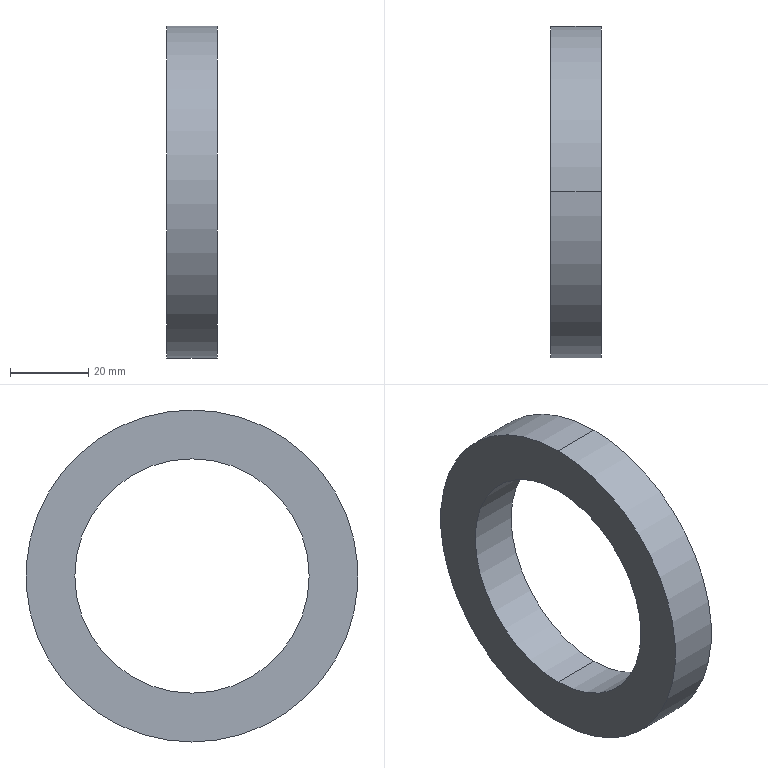Part | SolidWorks | features Extrusion 1 | 1 solid | 6 faces | box 13 x 85 x 85 mm | volume 37012 mm3 | cylinder 4 | plane 2 | commonest cylinder face diameters 60 x2 85 x2
STEP:
#1=CARTESIAN_POINT('',(13.,0.,30.));
#2=VERTEX_POINT('',#1);
#3=CARTESIAN_POINT('',(13.,0.,-30.));
#4=VERTEX_POINT('',#3);
#5=CARTESIAN_POINT('',(13.,0.,0.));
#6=DIRECTION('',(1.,0.,0.));
#7=DIRECTION('',(0.,0.,-1.));
#8=AXIS2_PLACEMENT_3D('',#5,#6,#7);
#9=CIRCLE('',#8,30.);
#10=EDGE_CURVE('',#2,#4,#9,.T.);
#11=ORIENTED_EDGE('',*,*,#10,.T.);
#12=CARTESIAN_POINT('',(0.,0.,-30.));
#13=VERTEX_POINT('',#12);
#14=CARTESIAN_POINT('',(13.,0.,-30.));
#15=DIRECTION('',(-1.,0.,0.));
#16=VECTOR('',#15,1000.);
#17=LINE('',#14,#16);
#18=EDGE_CURVE('',#4,#13,#17,.T.);
#19=ORIENTED_EDGE('',*,*,#18,.T.);
#20=CARTESIAN_POINT('',(0.,0.,30.));
#21=VERTEX_POINT('',#20);
#22=CARTESIAN_POINT('',(0.,0.,0.));
#23=DIRECTION('',(1.,0.,0.));
#24=DIRECTION('',(0.,0.,-1.));
#25=AXIS2_PLACEMENT_3D('',#22,#23,#24);
#26=CIRCLE('',#25,30.);
#27=EDGE_CURVE('',#21,#13,#26,.T.);
#28=ORIENTED_EDGE('',*,*,#27,.F.);
#29=CARTESIAN_POINT('',(13.,0.,30.));
#30=DIRECTION('',(-1.,0.,0.));
#31=VECTOR('',#30,1000.);
#32=LINE('',#29,#31);
#33=EDGE_CURVE('',#2,#21,#32,.T.);
#34=ORIENTED_EDGE('',*,*,#33,.F.);
#35=EDGE_LOOP('',(#11,#19,#28,#34));
#36=FACE_OUTER_BOUND('',#35,.T.);
#37=CARTESIAN_POINT('',(13.,0.,0.));
#38=DIRECTION('',(-1.,0.,0.));
#39=DIRECTION('',(0.,0.,1.));
#40=AXIS2_PLACEMENT_3D('',#37,#38,#39);
#41=CYLINDRICAL_SURFACE('',#40,30.);
#42=ADVANCED_FACE('',(#36),#41,.F.);
#43=CARTESIAN_POINT('',(13.,0.,-42.5));
#44=VERTEX_POINT('',#43);
#45=CARTESIAN_POINT('',(13.,0.,42.5));
#46=VERTEX_POINT('',#45);
#47=CARTESIAN_POINT('',(13.,0.,0.));
#48=DIRECTION('',(1.,0.,0.));
#49=DIRECTION('',(0.,0.,-1.));
#50=AXIS2_PLACEMENT_3D('',#47,#48,#49);
#51=CIRCLE('',#50,42.5);
#52=EDGE_CURVE('',#44,#46,#51,.T.);
#53=ORIENTED_EDGE('',*,*,#52,.F.);
#54=CARTESIAN_POINT('',(0.,0.,-42.5));
#55=VERTEX_POINT('',#54);
#56=CARTESIAN_POINT('',(13.,0.,-42.5));
#57=DIRECTION('',(-1.,0.,0.));
#58=VECTOR('',#57,1000.);
#59=LINE('',#56,#58);
#60=EDGE_CURVE('',#44,#55,#59,.T.);
#61=ORIENTED_EDGE('',*,*,#60,.T.);
#62=CARTESIAN_POINT('',(0.,0.,42.5));
#63=VERTEX_POINT('',#62);
#64=CARTESIAN_POINT('',(0.,0.,0.));
#65=DIRECTION('',(1.,0.,0.));
#66=DIRECTION('',(0.,0.,-1.));
#67=AXIS2_PLACEMENT_3D('',#64,#65,#66);
#68=CIRCLE('',#67,42.5);
#69=EDGE_CURVE('',#55,#63,#68,.T.);
#70=ORIENTED_EDGE('',*,*,#69,.T.);
#71=CARTESIAN_POINT('',(13.,0.,42.5));
#72=DIRECTION('',(-1.,0.,0.));
#73=VECTOR('',#72,1000.);
#74=LINE('',#71,#73);
#75=EDGE_CURVE('',#46,#63,#74,.T.);
#76=ORIENTED_EDGE('',*,*,#75,.F.);
#77=EDGE_LOOP('',(#53,#61,#70,#76));
#78=FACE_OUTER_BOUND('',#77,.T.);
#79=CARTESIAN_POINT('',(13.,0.,0.));
#80=DIRECTION('',(-1.,0.,0.));
#81=DIRECTION('',(0.,0.,1.));
#82=AXIS2_PLACEMENT_3D('',#79,#80,#81);
#83=CYLINDRICAL_SURFACE('',#82,42.5);
#84=ADVANCED_FACE('',(#78),#83,.T.);
#85=CARTESIAN_POINT('',(13.,0.,0.));
#86=DIRECTION('',(1.,0.,0.));
#87=DIRECTION('',(0.,0.,-1.));
#88=AXIS2_PLACEMENT_3D('',#85,#86,#87);
#89=CIRCLE('',#88,42.5);
#90=EDGE_CURVE('',#46,#44,#89,.T.);
#91=ORIENTED_EDGE('',*,*,#90,.T.);
#92=ORIENTED_EDGE('',*,*,#52,.T.);
#93=EDGE_LOOP('',(#91,#92));
#94=FACE_OUTER_BOUND('',#93,.T.);
#95=ORIENTED_EDGE('',*,*,#10,.F.);
#96=CARTESIAN_POINT('',(13.,0.,0.));
#97=DIRECTION('',(1.,0.,0.));
#98=DIRECTION('',(0.,0.,-1.));
#99=AXIS2_PLACEMENT_3D('',#96,#97,#98);
#100=CIRCLE('',#99,30.);
#101=EDGE_CURVE('',#4,#2,#100,.T.);
#102=ORIENTED_EDGE('',*,*,#101,.F.);
#103=EDGE_LOOP('',(#95,#102));
#104=FACE_BOUND('',#103,.T.);
#105=CARTESIAN_POINT('',(13.,0.,0.));
#106=DIRECTION('',(1.,0.,0.));
#107=DIRECTION('',(0.,0.,-1.));
#108=AXIS2_PLACEMENT_3D('',#105,#106,#107);
#109=PLANE('',#108);
#110=ADVANCED_FACE('',(#94,#104),#109,.T.);
#111=CARTESIAN_POINT('',(0.,0.,0.));
#112=DIRECTION('',(1.,0.,0.));
#113=DIRECTION('',(0.,0.,-1.));
#114=AXIS2_PLACEMENT_3D('',#111,#112,#113);
#115=CIRCLE('',#114,42.5);
#116=EDGE_CURVE('',#63,#55,#115,.T.);
#117=ORIENTED_EDGE('',*,*,#116,.F.);
#118=ORIENTED_EDGE('',*,*,#69,.F.);
#119=EDGE_LOOP('',(#117,#118));
#120=FACE_OUTER_BOUND('',#119,.T.);
#121=ORIENTED_EDGE('',*,*,#27,.T.);
#122=CARTESIAN_POINT('',(0.,0.,0.));
#123=DIRECTION('',(1.,0.,0.));
#124=DIRECTION('',(0.,0.,-1.));
#125=AXIS2_PLACEMENT_3D('',#122,#123,#124);
#126=CIRCLE('',#125,30.);
#127=EDGE_CURVE('',#13,#21,#126,.T.);
#128=ORIENTED_EDGE('',*,*,#127,.T.);
#129=EDGE_LOOP('',(#121,#128));
#130=FACE_BOUND('',#129,.T.);
#131=CARTESIAN_POINT('',(0.,0.,0.));
#132=DIRECTION('',(1.,0.,0.));
#133=DIRECTION('',(0.,0.,-1.));
#134=AXIS2_PLACEMENT_3D('',#131,#132,#133);
#135=PLANE('',#134);
#136=ADVANCED_FACE('',(#120,#130),#135,.F.);
#137=ORIENTED_EDGE('',*,*,#60,.F.);
#138=ORIENTED_EDGE('',*,*,#90,.F.);
#139=ORIENTED_EDGE('',*,*,#75,.T.);
#140=ORIENTED_EDGE('',*,*,#116,.T.);
#141=EDGE_LOOP('',(#137,#138,#139,#140));
#142=FACE_OUTER_BOUND('',#141,.T.);
#143=CARTESIAN_POINT('',(13.,0.,0.));
#144=DIRECTION('',(-1.,0.,0.));
#145=DIRECTION('',(0.,0.,1.));
#146=AXIS2_PLACEMENT_3D('',#143,#144,#145);
#147=CYLINDRICAL_SURFACE('',#146,42.5);
#148=ADVANCED_FACE('',(#142),#147,.T.);
#149=ORIENTED_EDGE('',*,*,#18,.F.);
#150=ORIENTED_EDGE('',*,*,#101,.T.);
#151=ORIENTED_EDGE('',*,*,#33,.T.);
#152=ORIENTED_EDGE('',*,*,#127,.F.);
#153=EDGE_LOOP('',(#149,#150,#151,#152));
#154=FACE_OUTER_BOUND('',#153,.T.);
#155=CARTESIAN_POINT('',(13.,0.,0.));
#156=DIRECTION('',(-1.,0.,0.));
#157=DIRECTION('',(0.,0.,1.));
#158=AXIS2_PLACEMENT_3D('',#155,#156,#157);
#159=CYLINDRICAL_SURFACE('',#158,30.);
#160=ADVANCED_FACE('',(#154),#159,.F.);
#161=CLOSED_SHELL('',(#42,#84,#110,#136,#148,#160));
#162=MANIFOLD_SOLID_BREP('',#161);
#163=CARTESIAN_POINT('',(0.,0.,0.));
#164=DIRECTION('',(0.,0.,1.));
#165=DIRECTION('',(1.,0.,0.));
#166=AXIS2_PLACEMENT_3D('',#163,#164,#165);
#167=(LENGTH_UNIT()NAMED_UNIT(*)SI_UNIT(.MILLI.,.METRE.));
#168=UNCERTAINTY_MEASURE_WITH_UNIT(LENGTH_MEASURE(0.00001),#167,'','');
#169=(NAMED_UNIT(*)PLANE_ANGLE_UNIT()SI_UNIT($,.RADIAN.));
#170=(NAMED_UNIT(*)SI_UNIT($,.STERADIAN.)SOLID_ANGLE_UNIT());
#171=(GEOMETRIC_REPRESENTATION_CONTEXT(3)GLOBAL_UNCERTAINTY_ASSIGNED_CONTEXT((#168))GLOBAL_UNIT_ASSIGNED_CONTEXT((#167,#169,#170))REPRESENTATION_CONTEXT('',''));
#172=ADVANCED_BREP_SHAPE_REPRESENTATION('',(#162,#166),#171);